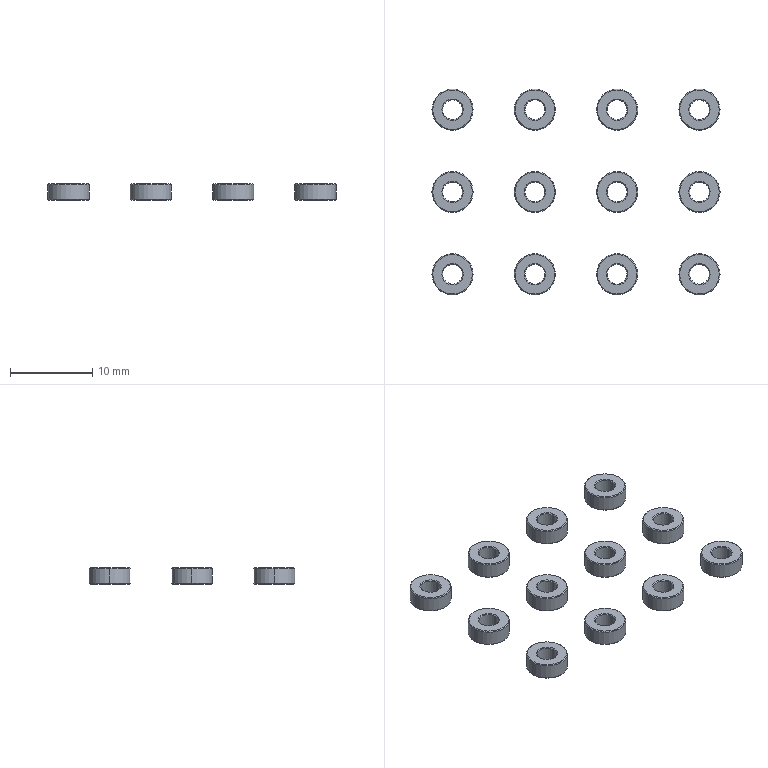CAM job | NX | 3-axis milling, drilling | part box 35 x 25 x 2 mm | stock box 35 x 25 x 2 mm
Tools:
number,name,description,diameter,corner_radius,flute_length,length,flutes
7,D6A45,Milling Tool-5 Parameters,6.0,0.0,50.0,75.0,2
14,2.4ZT,Drilling Tool,2.4,0.0,35.0,50.0,2
4,D4,Milling Tool-5 Parameters,4.0,0.0,50.0,75.0,2
Operations:
program,operation,operation_type,tool,method,geometry_group,spindle_rpm,surface_speed,feed_per_tooth,feed_cut,feed_plunge,cut_length_mm,path_length_mm,cut_time_min,machine_time_min
1,DRILLING,Operation,D6A45,METHOD,A,5000.0,94.0,0.025,250.0,0.0,51.6,311.043,0.2064,0.2323
1,DRILLING_COPY,Operation,2.4ZT,METHOD,A,2000.0,15.0,0.0375,150.0,0.0,86.652,381.148,0.5777,0.6071
1,ZLEVEL_PROFILE,ZLevelMilling,D4,METHOD,A,9500.0,298.0,0.1316,2500.0,1000.0,2352.814,3765.181,1.186,1.327
1,ZLEVEL_PROFILE_1_COPY,ZLevelMilling,D6A45,METHOD,A,9500.0,179.0,0.0658,1250.0,100.0,427.847,2165.819,0.3423,0.5161
1,ZLEVEL_PROFILE_COPY,ZLevelMilling,D4,METHOD,A,9500.0,298.0,0.0526,1000.0,1000.0,1502.05,2965.022,1.502,1.648